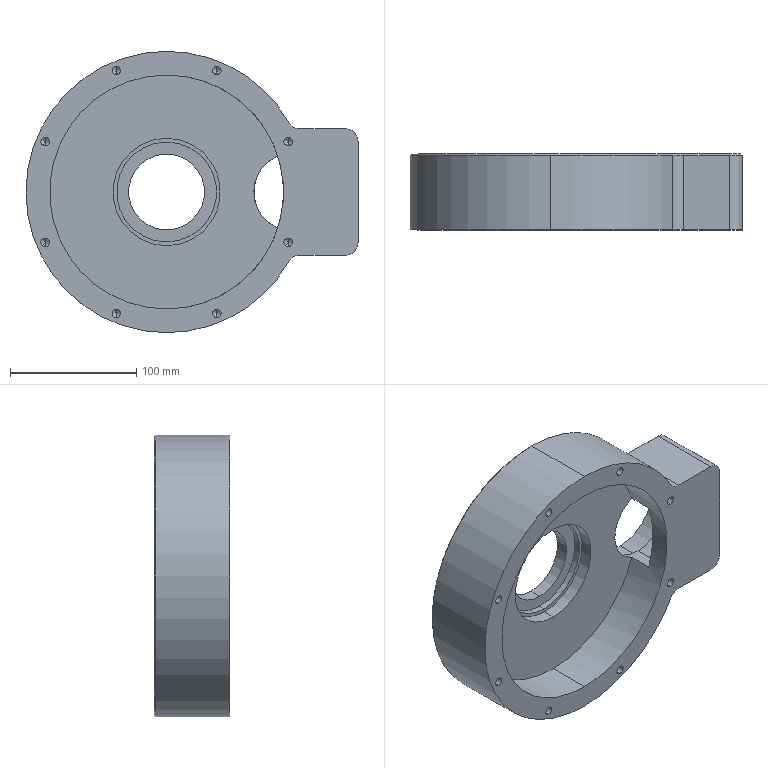Part | SolidWorks | features HoleWzd 5, ICE 5, Chamfer 1, Cut 1, Fillet 1, Revolution 1 | 1 solid | 195 faces | box 262.631 x 60 x 222.5 mm | volume 1391855 mm3 | cylinder 97 | cone 85 | plane 13 | commonest cylinder face diameters 6.8 x32 5 x24 3.3 x12 4.2 x10 20 x4 222.5 x3